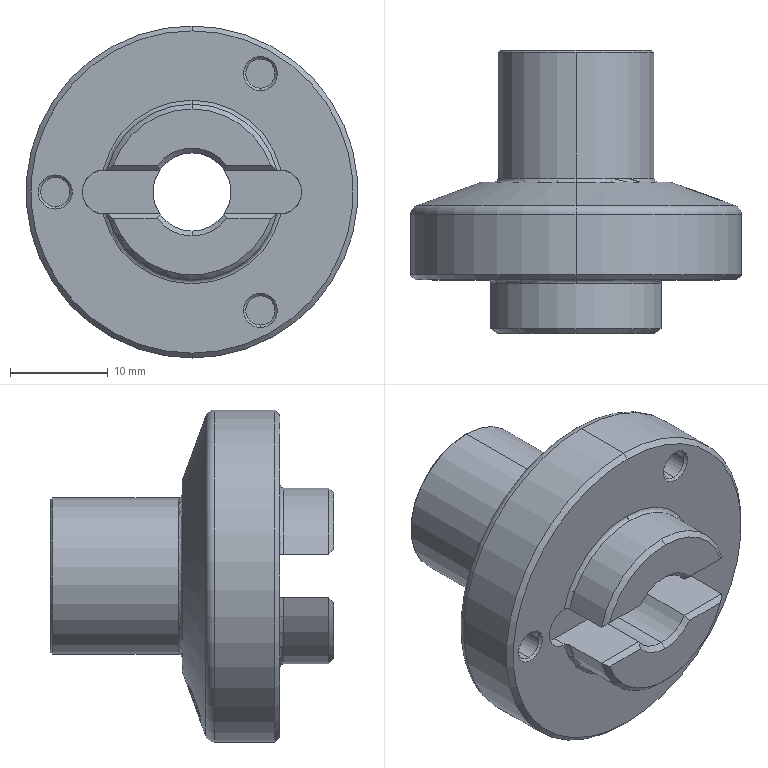Part | STEP file | QCTHA0834-14_01^qctha0834-14_FBDS-CS | 1 solid | 150 faces | box 34 x 29 x 34 mm | volume 9325 mm3 | plane 55 | cone 33 | spline 32 | cylinder 21 | torus 9 | commonest cylinder face diameters 3 x6 18 x3 4.5 x2 8 x2 12.5 x2 16 x2